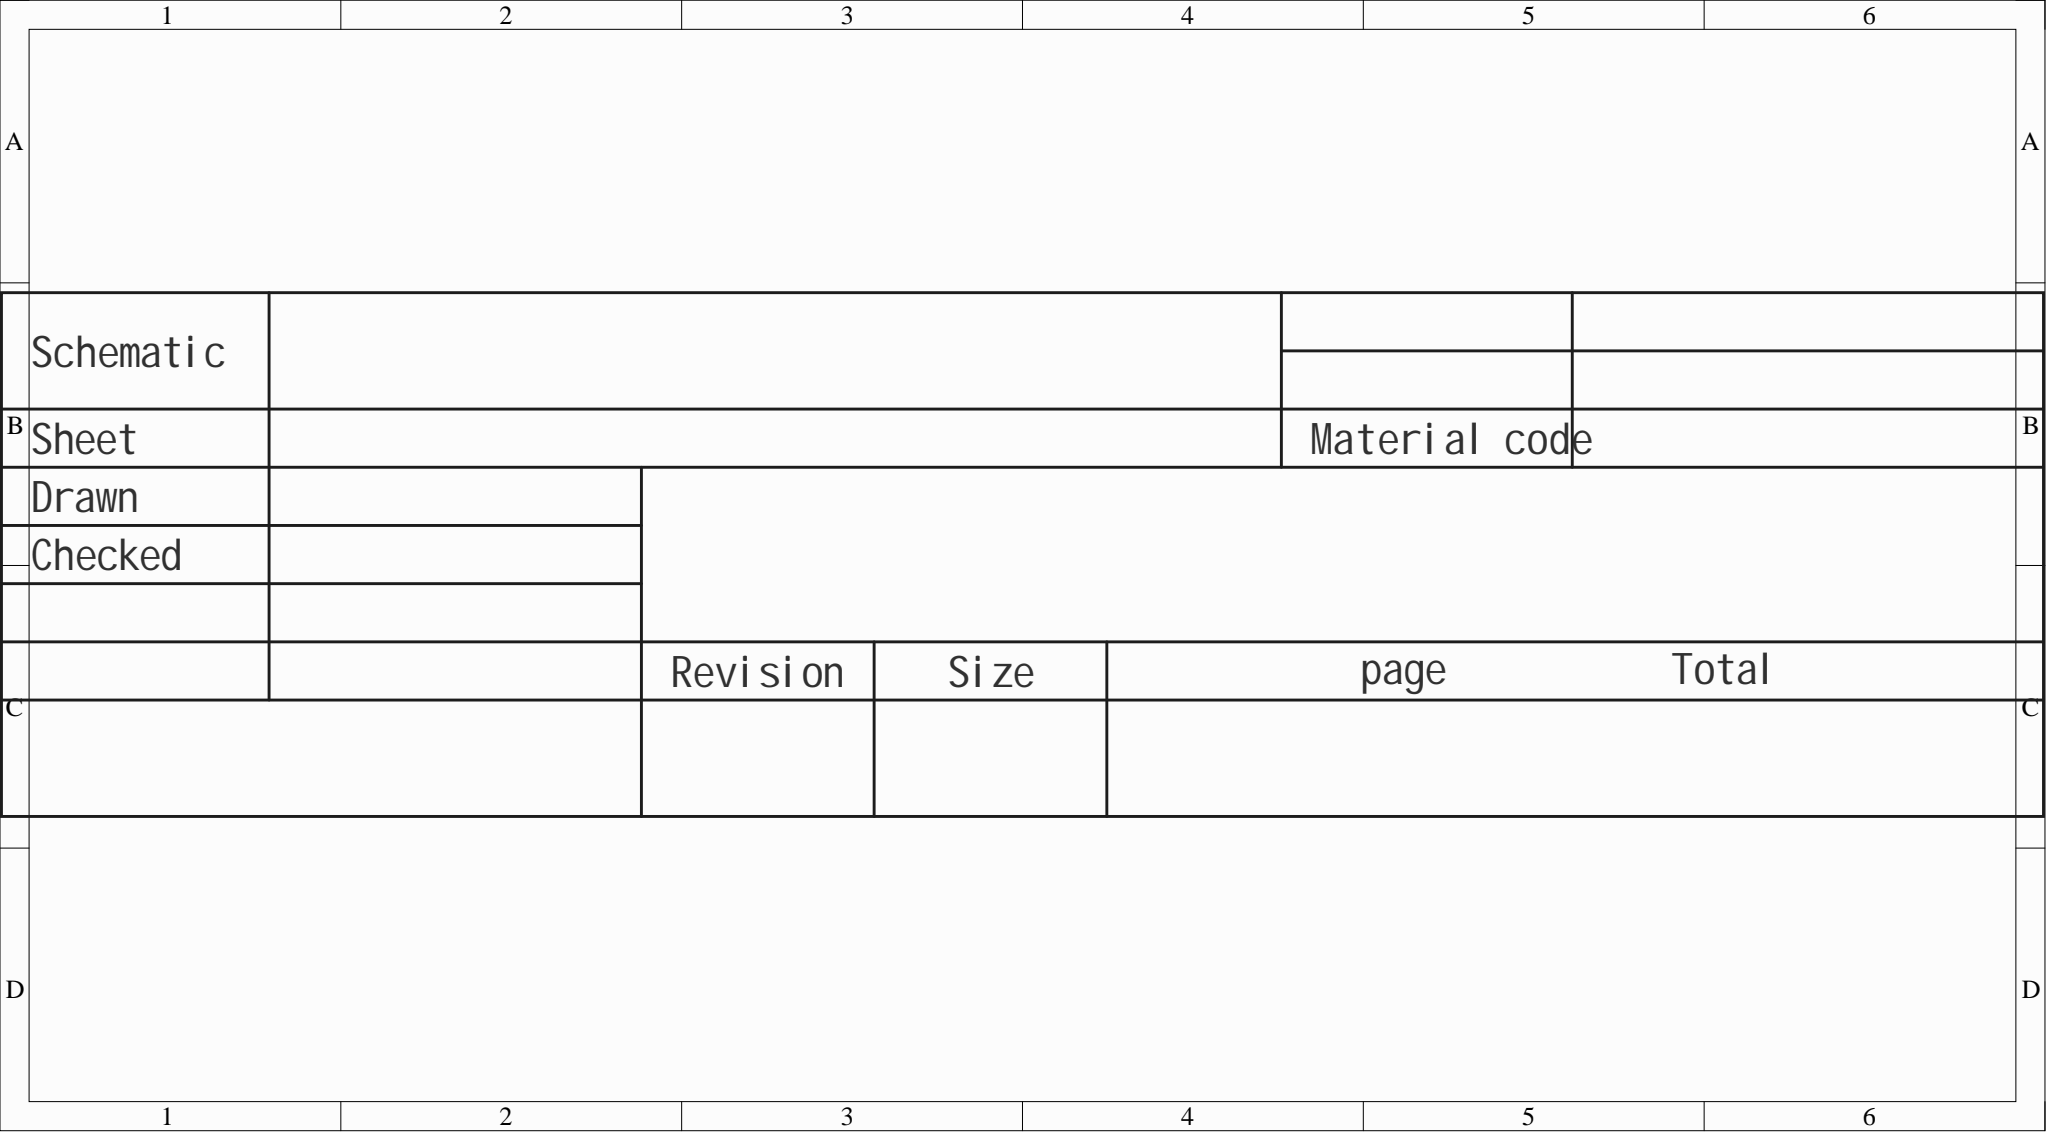Circuit board | Altium Designer | 40 parts | 31 nets
Bill of materials:
Comment,Description,Designator,Footprint,LibRef,Quantity
"22pF","Capacitance: 30pF; tolerance: ±5%; rated voltage: 50V; temperature coefficient: C0G;","C5, C6","CAP-TH_L3.6-W2.3-P5.00-D0.5","K300J10C0GF5UH5","2"
"100pF","","C7","C0603","CAP_0603","1"
"100nF","","C8, C9","C0603","CAP_0603","2"
"","Diode configuration: single; DC reverse voltage (Vr): 1kV; average rectified current (Io): 1A; forward voltage (Vf): 1.1V@1A; reverse current (Ir): 10A@1kV;","D1, D2, D3, D4, D5, D6, D7, D8","SOD-123FL_L2.7-W1.8-LS3.8-RD","1N4007","8"
"","","LED1","LED_0603","LED_0603-R","1"
"LCM1027A2445F","Type: flat vibration motor; rated voltage: 3V; rated speed: 10000rpm; rotation direction: CW; CCW;","MOT1, MOT2, MOT3","VIBRATING-MOTOR-SMD_WELDING","LCM1027A2445F","3"
"","","Q1","S8550P_SOT","S8550_SOT_PNP","1"
"10kΩ","","R39","Res_1/8W","Res_AXIAL-1/8W","1"
"5.1K","","R43, R44","R0603","Res_0603","2"
"1K","","R45, R54, R56","R0603","Res_0603","3"
"10kΩ","Resistance: 10kΩ; tolerance: ±25%; power: 100mW;","R47, R51","RES-ADJ-SMD_RM065-V1","RM065-103(10K)","2"
"10K","","R48, R50, R53, R55","R0603","Res_0603","4"
"100K","","R49","R0603","Res_0603","1"
"47K","","R52","R0603","Res_0603","1"
"Tactile switch, 6*6*5 plastic head, 260G, travel 0.25mm, through-hole 2-pin","","SW11","KEY-TH_2P-L6.0-W6.0-P5.00","轻触开关,6*6*5塑头,260G,行程0.25mm,直插中2脚","1"
"12MHz","Frequency: 12MHz; frequency tolerance at room temp: ±30ppm; external load capacitance: -; frequency stability (full temp): ±50ppm;","U2","HC-49US_L11.0-W4.6-P4.88","ECS-120-S-4","1"
"AT89C51","CPU core: 51 series; program memory capacity: 61KB; RAM total capacity: 1.25KB; GPIO port count: 35; operating voltage range: 3.5V~5.5V; CPU max clock: -; program memory type: FLASH;","U3","DIP-40_L52.3-W13.9-P2.54-LS15.2-BL","STC89C516RD+40I-PDIP40","1"
"L298N","Supply voltage: 4.5V~7V; features: overcurrent protection (OCP); overtemperature protection (OPT);","U11","MULTIWATT-15_L19.6-W5.0-P1.27-L","L298N_C19922","1"
"LM393M","","U12","SOIC-8_L4.9-W3.9-P1.27-LS6.0-BL","LM393M_C258241","1"
"XL-ITR9707","Plug-in, through-beam photoelectric switch, high reliability, high radiant intensity, low-voltage drive, fast response, high sensitivity, automatic sensor","U13, U14","OPTO-TH_4P-P2.54-XL-ITR9608","XL-ITR9707","2"
"TYPE_C_SMD_6P","","USB1","TYPE-C-SMD_TYPE-C-6P","TYPE_C_SMD_6P","1"
Netlist (Protel format):
[
C5
CAP-TH_L3.6-W2.3-P5.00-D0.5
22pF



]
[
C6
CAP-TH_L3.6-W2.3-P5.00-D0.5
22pF



]
[
C7
C0603
100pF



]
[
C8
C0603
100nF



]
[
C9
C0603
100nF



]
[
D1
SOD-123FL_L2.7-W1.8-LS3.8-RD




]
[
D2
SOD-123FL_L2.7-W1.8-LS3.8-RD




]
[
D3
SOD-123FL_L2.7-W1.8-LS3.8-RD




]
[
D4
SOD-123FL_L2.7-W1.8-LS3.8-RD




]
[
D5
SOD-123FL_L2.7-W1.8-LS3.8-RD




]
[
D6
SOD-123FL_L2.7-W1.8-LS3.8-RD




]
[
D7
SOD-123FL_L2.7-W1.8-LS3.8-RD




]
[
D8
SOD-123FL_L2.7-W1.8-LS3.8-RD




]
[
LED1
LED_0603




]
[
MOT1
VIBRATING-MOTOR-SMD_WELDING
LCM1027A2445F



]
[
MOT2
VIBRATING-MOTOR-SMD_WELDING
LCM1027A2445F



]
[
MOT3
VIBRATING-MOTOR-SMD_WELDING
LCM1027A2445F



]
[
Q1
S8550P_SOT




]
[
R39
Res_1/8W
10kΩ



]
[
R43
R0603
5.1K



]
[
R44
R0603
5.1K



]
[
R45
R0603
1K



]
[
R47
RES-ADJ-SMD_RM065-V1
10kΩ



]
[
R48
R0603
10K



]
[
R49
R0603
100K



]
[
R50
R0603
10K



]
[
R51
RES-ADJ-SMD_RM065-V1
10kΩ



]
[
R52
R0603
47K



]
[
R53
R0603
10K



]
[
R54
R0603
1K



]
[
R55
R0603
10K



]
[
R56
R0603
1K



]
[
SW11
KEY-TH_2P-L6.0-W6.0-P5.00
Tactile switch, 6*6*5 plastic head, 260G, travel 0.25mm, through-hole 2-pin



]
[
U2
HC-49US_L11.0-W4.6-P4.88
12MHz



]
[
U3
DIP-40_L52.3-W13.9-P2.54-LS15.2-BL
AT89C51



]
[
U11
MULTIWATT-15_L19.6-W5.0-P1.27-L
L298N



]
[
U12
SOIC-8_L4.9-W3.9-P1.27-LS6.0-BL
LM393M



]
[
U13
OPTO-TH_4P-P2.54-XL-ITR9608
XL-ITR9707



]
[
U14
OPTO-TH_4P-P2.54-XL-ITR9608
XL-ITR9707



]
[
USB1
TYPE-C-SMD_TYPE-C-6P
TYPE_C_SMD_6P



]
(
VCC
C7-2
C8-2
LED1-2
MOT1-2
R47-1
R48-2
R49-2
R50-2
R51-1
R53-2
R55-2
SW11-1
U3-40
U12-8
U14-2
USB1-A9
USB1-B9
)
(
NetU14_1
U14-1
U14-4
)
(
NetR53_1
R53-1
R54-2
U12-7
)
(
NetR52_2
R52-2
U12-5
U14-3
)
(
NetR51_2
R51-2
U12-6
)
(
NetR49_1
R49-1
U13-1
)
(
NetR48_1
R48-1
U12-3
)
(
NetR45_1
R45-1
U3-32
)
(
NetR44_2
R44-2
USB1-B5
)
(
NetR43_2
R43-2
USB1-A5
)
(
NetQ1_1
Q1-1
R45-2
)
(
NetMOT1_1
MOT1-1
Q1-2
)
(
NetLED1_1
LED1-1
R56-2
)
(
NetD4_2
D4-2
D8-1
MOT3-1
U11-14
)
(
NetD3_2
D3-2
D7-1
MOT3-2
U11-13
)
(
NetD2_2
D2-2
D6-1
MOT2-1
U11-3
)
(
NetD1_2
D1-2
D5-1
MOT2-2
U11-2
)
(
NetC9_2
C9-2
R47-2
U12-2
U13-4
)
(
NetC7_1
C7-1
R39-2
SW11-2
U3-9
)
(
NetC6_2
C6-2
U2-2
U3-19
)
(
NetC5_2
C5-2
U2-1
U3-18
)
(
IN4
U3-1
U11-12
)
(
IN3
U3-2
U11-10
)
(
IN2
U3-4
U11-7
)
(
IN1
U3-5
U11-5
)
(
GND
C5-1
C6-1
C8-1
C9-1
D5-2
D6-2
D7-2
D8-2
Q1-3
R39-1
R43-1
R44-1
R47-3
R51-3
R52-1
R55-1
R56-1
U3-20
U11-1
U11-8
U11-15
U12-4
U13-2
U13-3
USB1-7
USB1-A12
USB1-B12
)
(
FANGDIELUO
R54-1
U3-22
)
(
EB
U3-3
U11-11
)
(
EA
U3-6
U11-6
)
(
BIZHANG
R50-1
U3-21
U12-1
)
(
12V
D1-1
D2-1
D3-1
D4-1
U11-4
)